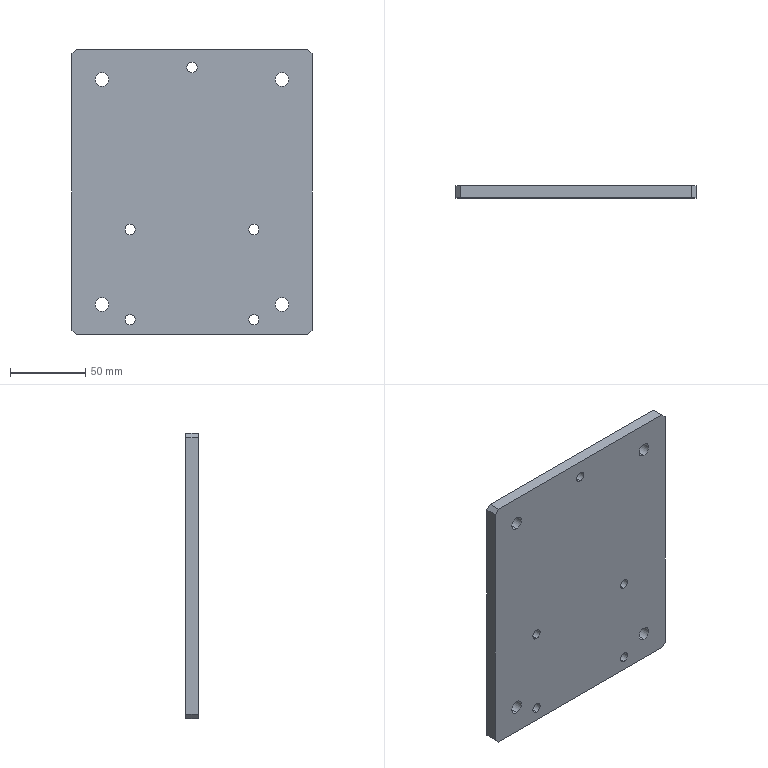Part | SolidWorks | features HoleWzd 3, Chamfer 1, Extrusion 1 | 1 solid | 28 faces | box 160 x 8 x 190 mm | volume 239568 mm3 | cylinder 18 | plane 10 | commonest cylinder face diameters 6.8 x10 9 x8
STEP:
#1=CARTESIAN_POINT('',(0.,4.,86.4));
#2=VERTEX_POINT('',#1);
#3=CARTESIAN_POINT('',(0.,4.,79.6));
#4=VERTEX_POINT('',#3);
#5=CARTESIAN_POINT('',(0.,4.,83.));
#6=DIRECTION('',(0.,-1.,0.));
#7=DIRECTION('',(0.,0.,-1.));
#8=AXIS2_PLACEMENT_3D('',#5,#6,#7);
#9=CIRCLE('',#8,3.4);
#10=EDGE_CURVE('',#2,#4,#9,.T.);
#11=ORIENTED_EDGE('',*,*,#10,.F.);
#12=CARTESIAN_POINT('',(0.,-4.,86.4));
#13=VERTEX_POINT('',#12);
#14=CARTESIAN_POINT('',(0.,-4.,86.4));
#15=DIRECTION('',(0.,-1.,0.));
#16=VECTOR('',#15,1000.);
#17=LINE('',#14,#16);
#18=EDGE_CURVE('',#2,#13,#17,.T.);
#19=ORIENTED_EDGE('',*,*,#18,.T.);
#20=CARTESIAN_POINT('',(0.,-4.,79.6));
#21=VERTEX_POINT('',#20);
#22=CARTESIAN_POINT('',(0.,-4.,83.));
#23=DIRECTION('',(0.,-1.,0.));
#24=DIRECTION('',(0.,0.,-1.));
#25=AXIS2_PLACEMENT_3D('',#22,#23,#24);
#26=CIRCLE('',#25,3.4);
#27=EDGE_CURVE('',#13,#21,#26,.T.);
#28=ORIENTED_EDGE('',*,*,#27,.T.);
#29=CARTESIAN_POINT('',(0.,-4.,79.6));
#30=DIRECTION('',(0.,-1.,0.));
#31=VECTOR('',#30,1000.);
#32=LINE('',#29,#31);
#33=EDGE_CURVE('',#4,#21,#32,.T.);
#34=ORIENTED_EDGE('',*,*,#33,.F.);
#35=EDGE_LOOP('',(#11,#19,#28,#34));
#36=FACE_OUTER_BOUND('',#35,.T.);
#37=CARTESIAN_POINT('',(0.,-4.,83.));
#38=DIRECTION('',(0.,-1.,0.));
#39=DIRECTION('',(0.,0.,-1.));
#40=AXIS2_PLACEMENT_3D('',#37,#38,#39);
#41=CYLINDRICAL_SURFACE('',#40,3.4);
#42=ADVANCED_FACE('',(#36),#41,.F.);
#43=CARTESIAN_POINT('',(41.25,4.,-21.6));
#44=VERTEX_POINT('',#43);
#45=CARTESIAN_POINT('',(41.25,4.,-28.4));
#46=VERTEX_POINT('',#45);
#47=CARTESIAN_POINT('',(41.25,4.,-25.));
#48=DIRECTION('',(0.,-1.,0.));
#49=DIRECTION('',(0.,0.,-1.));
#50=AXIS2_PLACEMENT_3D('',#47,#48,#49);
#51=CIRCLE('',#50,3.4);
#52=EDGE_CURVE('',#44,#46,#51,.T.);
#53=ORIENTED_EDGE('',*,*,#52,.F.);
#54=CARTESIAN_POINT('',(41.25,-4.,-21.6));
#55=VERTEX_POINT('',#54);
#56=CARTESIAN_POINT('',(41.25,-4.,-21.6));
#57=DIRECTION('',(0.,-1.,0.));
#58=VECTOR('',#57,1000.);
#59=LINE('',#56,#58);
#60=EDGE_CURVE('',#44,#55,#59,.T.);
#61=ORIENTED_EDGE('',*,*,#60,.T.);
#62=CARTESIAN_POINT('',(41.25,-4.,-28.4));
#63=VERTEX_POINT('',#62);
#64=CARTESIAN_POINT('',(41.25,-4.,-25.));
#65=DIRECTION('',(0.,-1.,0.));
#66=DIRECTION('',(0.,0.,-1.));
#67=AXIS2_PLACEMENT_3D('',#64,#65,#66);
#68=CIRCLE('',#67,3.4);
#69=EDGE_CURVE('',#55,#63,#68,.T.);
#70=ORIENTED_EDGE('',*,*,#69,.T.);
#71=CARTESIAN_POINT('',(41.25,-4.,-28.4));
#72=DIRECTION('',(0.,-1.,0.));
#73=VECTOR('',#72,1000.);
#74=LINE('',#71,#73);
#75=EDGE_CURVE('',#46,#63,#74,.T.);
#76=ORIENTED_EDGE('',*,*,#75,.F.);
#77=EDGE_LOOP('',(#53,#61,#70,#76));
#78=FACE_OUTER_BOUND('',#77,.T.);
#79=CARTESIAN_POINT('',(41.25,-4.,-25.));
#80=DIRECTION('',(0.,-1.,0.));
#81=DIRECTION('',(0.,0.,-1.));
#82=AXIS2_PLACEMENT_3D('',#79,#80,#81);
#83=CYLINDRICAL_SURFACE('',#82,3.4);
#84=ADVANCED_FACE('',(#78),#83,.F.);
#85=CARTESIAN_POINT('',(41.25,4.,-81.6));
#86=VERTEX_POINT('',#85);
#87=CARTESIAN_POINT('',(41.25,4.,-88.4));
#88=VERTEX_POINT('',#87);
#89=CARTESIAN_POINT('',(41.25,4.,-85.));
#90=DIRECTION('',(0.,-1.,0.));
#91=DIRECTION('',(0.,0.,-1.));
#92=AXIS2_PLACEMENT_3D('',#89,#90,#91);
#93=CIRCLE('',#92,3.4);
#94=EDGE_CURVE('',#86,#88,#93,.T.);
#95=ORIENTED_EDGE('',*,*,#94,.F.);
#96=CARTESIAN_POINT('',(41.25,-4.,-81.6));
#97=VERTEX_POINT('',#96);
#98=CARTESIAN_POINT('',(41.25,-4.,-81.6));
#99=DIRECTION('',(0.,-1.,0.));
#100=VECTOR('',#99,1000.);
#101=LINE('',#98,#100);
#102=EDGE_CURVE('',#86,#97,#101,.T.);
#103=ORIENTED_EDGE('',*,*,#102,.T.);
#104=CARTESIAN_POINT('',(41.25,-4.,-88.4));
#105=VERTEX_POINT('',#104);
#106=CARTESIAN_POINT('',(41.25,-4.,-85.));
#107=DIRECTION('',(0.,-1.,0.));
#108=DIRECTION('',(0.,0.,-1.));
#109=AXIS2_PLACEMENT_3D('',#106,#107,#108);
#110=CIRCLE('',#109,3.4);
#111=EDGE_CURVE('',#97,#105,#110,.T.);
#112=ORIENTED_EDGE('',*,*,#111,.T.);
#113=CARTESIAN_POINT('',(41.25,-4.,-88.4));
#114=DIRECTION('',(0.,-1.,0.));
#115=VECTOR('',#114,1000.);
#116=LINE('',#113,#115);
#117=EDGE_CURVE('',#88,#105,#116,.T.);
#118=ORIENTED_EDGE('',*,*,#117,.F.);
#119=EDGE_LOOP('',(#95,#103,#112,#118));
#120=FACE_OUTER_BOUND('',#119,.T.);
#121=CARTESIAN_POINT('',(41.25,-4.,-85.));
#122=DIRECTION('',(0.,-1.,0.));
#123=DIRECTION('',(0.,0.,-1.));
#124=AXIS2_PLACEMENT_3D('',#121,#122,#123);
#125=CYLINDRICAL_SURFACE('',#124,3.4);
#126=ADVANCED_FACE('',(#120),#125,.F.);
#127=CARTESIAN_POINT('',(-41.25,4.,-81.6));
#128=VERTEX_POINT('',#127);
#129=CARTESIAN_POINT('',(-41.25,4.,-88.4));
#130=VERTEX_POINT('',#129);
#131=CARTESIAN_POINT('',(-41.25,4.,-85.));
#132=DIRECTION('',(0.,-1.,0.));
#133=DIRECTION('',(0.,0.,-1.));
#134=AXIS2_PLACEMENT_3D('',#131,#132,#133);
#135=CIRCLE('',#134,3.4);
#136=EDGE_CURVE('',#128,#130,#135,.T.);
#137=ORIENTED_EDGE('',*,*,#136,.F.);
#138=CARTESIAN_POINT('',(-41.25,-4.,-81.6));
#139=VERTEX_POINT('',#138);
#140=CARTESIAN_POINT('',(-41.25,-4.,-81.6));
#141=DIRECTION('',(0.,-1.,0.));
#142=VECTOR('',#141,1000.);
#143=LINE('',#140,#142);
#144=EDGE_CURVE('',#128,#139,#143,.T.);
#145=ORIENTED_EDGE('',*,*,#144,.T.);
#146=CARTESIAN_POINT('',(-41.25,-4.,-88.4));
#147=VERTEX_POINT('',#146);
#148=CARTESIAN_POINT('',(-41.25,-4.,-85.));
#149=DIRECTION('',(0.,-1.,0.));
#150=DIRECTION('',(0.,0.,-1.));
#151=AXIS2_PLACEMENT_3D('',#148,#149,#150);
#152=CIRCLE('',#151,3.4);
#153=EDGE_CURVE('',#139,#147,#152,.T.);
#154=ORIENTED_EDGE('',*,*,#153,.T.);
#155=CARTESIAN_POINT('',(-41.25,-4.,-88.4));
#156=DIRECTION('',(0.,-1.,0.));
#157=VECTOR('',#156,1000.);
#158=LINE('',#155,#157);
#159=EDGE_CURVE('',#130,#147,#158,.T.);
#160=ORIENTED_EDGE('',*,*,#159,.F.);
#161=EDGE_LOOP('',(#137,#145,#154,#160));
#162=FACE_OUTER_BOUND('',#161,.T.);
#163=CARTESIAN_POINT('',(-41.25,-4.,-85.));
#164=DIRECTION('',(0.,-1.,0.));
#165=DIRECTION('',(0.,0.,-1.));
#166=AXIS2_PLACEMENT_3D('',#163,#164,#165);
#167=CYLINDRICAL_SURFACE('',#166,3.4);
#168=ADVANCED_FACE('',(#162),#167,.F.);
#169=CARTESIAN_POINT('',(-41.25,4.,-21.6));
#170=VERTEX_POINT('',#169);
#171=CARTESIAN_POINT('',(-41.25,4.,-28.4));
#172=VERTEX_POINT('',#171);
#173=CARTESIAN_POINT('',(-41.25,4.,-25.));
#174=DIRECTION('',(0.,-1.,0.));
#175=DIRECTION('',(0.,0.,-1.));
#176=AXIS2_PLACEMENT_3D('',#173,#174,#175);
#177=CIRCLE('',#176,3.4);
#178=EDGE_CURVE('',#170,#172,#177,.T.);
#179=ORIENTED_EDGE('',*,*,#178,.F.);
#180=CARTESIAN_POINT('',(-41.25,-4.,-21.6));
#181=VERTEX_POINT('',#180);
#182=CARTESIAN_POINT('',(-41.25,-4.,-21.6));
#183=DIRECTION('',(0.,-1.,0.));
#184=VECTOR('',#183,1000.);
#185=LINE('',#182,#184);
#186=EDGE_CURVE('',#170,#181,#185,.T.);
#187=ORIENTED_EDGE('',*,*,#186,.T.);
#188=CARTESIAN_POINT('',(-41.25,-4.,-28.4));
#189=VERTEX_POINT('',#188);
#190=CARTESIAN_POINT('',(-41.25,-4.,-25.));
#191=DIRECTION('',(0.,-1.,0.));
#192=DIRECTION('',(0.,0.,-1.));
#193=AXIS2_PLACEMENT_3D('',#190,#191,#192);
#194=CIRCLE('',#193,3.4);
#195=EDGE_CURVE('',#181,#189,#194,.T.);
#196=ORIENTED_EDGE('',*,*,#195,.T.);
#197=CARTESIAN_POINT('',(-41.25,-4.,-28.4));
#198=DIRECTION('',(0.,-1.,0.));
#199=VECTOR('',#198,1000.);
#200=LINE('',#197,#199);
#201=EDGE_CURVE('',#172,#189,#200,.T.);
#202=ORIENTED_EDGE('',*,*,#201,.F.);
#203=EDGE_LOOP('',(#179,#187,#196,#202));
#204=FACE_OUTER_BOUND('',#203,.T.);
#205=CARTESIAN_POINT('',(-41.25,-4.,-25.));
#206=DIRECTION('',(0.,-1.,0.));
#207=DIRECTION('',(0.,0.,-1.));
#208=AXIS2_PLACEMENT_3D('',#205,#206,#207);
#209=CYLINDRICAL_SURFACE('',#208,3.4);
#210=ADVANCED_FACE('',(#204),#209,.F.);
#211=CARTESIAN_POINT('',(60.,4.,79.5));
#212=VERTEX_POINT('',#211);
#213=CARTESIAN_POINT('',(60.,4.,70.5));
#214=VERTEX_POINT('',#213);
#215=CARTESIAN_POINT('',(60.,4.,75.));
#216=DIRECTION('',(0.,-1.,0.));
#217=DIRECTION('',(0.,0.,-1.));
#218=AXIS2_PLACEMENT_3D('',#215,#216,#217);
#219=CIRCLE('',#218,4.5);
#220=EDGE_CURVE('',#212,#214,#219,.T.);
#221=ORIENTED_EDGE('',*,*,#220,.F.);
#222=CARTESIAN_POINT('',(60.,-4.,79.5));
#223=VERTEX_POINT('',#222);
#224=CARTESIAN_POINT('',(60.,-4.,79.5));
#225=DIRECTION('',(0.,-1.,0.));
#226=VECTOR('',#225,1000.);
#227=LINE('',#224,#226);
#228=EDGE_CURVE('',#212,#223,#227,.T.);
#229=ORIENTED_EDGE('',*,*,#228,.T.);
#230=CARTESIAN_POINT('',(60.,-4.,70.5));
#231=VERTEX_POINT('',#230);
#232=CARTESIAN_POINT('',(60.,-4.,75.));
#233=DIRECTION('',(0.,-1.,0.));
#234=DIRECTION('',(0.,0.,-1.));
#235=AXIS2_PLACEMENT_3D('',#232,#233,#234);
#236=CIRCLE('',#235,4.5);
#237=EDGE_CURVE('',#223,#231,#236,.T.);
#238=ORIENTED_EDGE('',*,*,#237,.T.);
#239=CARTESIAN_POINT('',(60.,-4.,70.5));
#240=DIRECTION('',(0.,-1.,0.));
#241=VECTOR('',#240,1000.);
#242=LINE('',#239,#241);
#243=EDGE_CURVE('',#214,#231,#242,.T.);
#244=ORIENTED_EDGE('',*,*,#243,.F.);
#245=EDGE_LOOP('',(#221,#229,#238,#244));
#246=FACE_OUTER_BOUND('',#245,.T.);
#247=CARTESIAN_POINT('',(60.,-4.,75.));
#248=DIRECTION('',(0.,-1.,0.));
#249=DIRECTION('',(0.,0.,-1.));
#250=AXIS2_PLACEMENT_3D('',#247,#248,#249);
#251=CYLINDRICAL_SURFACE('',#250,4.5);
#252=ADVANCED_FACE('',(#246),#251,.F.);
#253=CARTESIAN_POINT('',(-60.,4.,79.5));
#254=VERTEX_POINT('',#253);
#255=CARTESIAN_POINT('',(-60.,4.,70.5));
#256=VERTEX_POINT('',#255);
#257=CARTESIAN_POINT('',(-60.,4.,75.));
#258=DIRECTION('',(0.,-1.,0.));
#259=DIRECTION('',(0.,0.,-1.));
#260=AXIS2_PLACEMENT_3D('',#257,#258,#259);
#261=CIRCLE('',#260,4.5);
#262=EDGE_CURVE('',#254,#256,#261,.T.);
#263=ORIENTED_EDGE('',*,*,#262,.F.);
#264=CARTESIAN_POINT('',(-60.,-4.,79.5));
#265=VERTEX_POINT('',#264);
#266=CARTESIAN_POINT('',(-60.,-4.,79.5));
#267=DIRECTION('',(0.,-1.,0.));
#268=VECTOR('',#267,1000.);
#269=LINE('',#266,#268);
#270=EDGE_CURVE('',#254,#265,#269,.T.);
#271=ORIENTED_EDGE('',*,*,#270,.T.);
#272=CARTESIAN_POINT('',(-60.,-4.,70.5));
#273=VERTEX_POINT('',#272);
#274=CARTESIAN_POINT('',(-60.,-4.,75.));
#275=DIRECTION('',(0.,-1.,0.));
#276=DIRECTION('',(0.,0.,-1.));
#277=AXIS2_PLACEMENT_3D('',#274,#275,#276);
#278=CIRCLE('',#277,4.5);
#279=EDGE_CURVE('',#265,#273,#278,.T.);
#280=ORIENTED_EDGE('',*,*,#279,.T.);
#281=CARTESIAN_POINT('',(-60.,-4.,70.5));
#282=DIRECTION('',(0.,-1.,0.));
#283=VECTOR('',#282,1000.);
#284=LINE('',#281,#283);
#285=EDGE_CURVE('',#256,#273,#284,.T.);
#286=ORIENTED_EDGE('',*,*,#285,.F.);
#287=EDGE_LOOP('',(#263,#271,#280,#286));
#288=FACE_OUTER_BOUND('',#287,.T.);
#289=CARTESIAN_POINT('',(-60.,-4.,75.));
#290=DIRECTION('',(0.,-1.,0.));
#291=DIRECTION('',(0.,0.,-1.));
#292=AXIS2_PLACEMENT_3D('',#289,#290,#291);
#293=CYLINDRICAL_SURFACE('',#292,4.5);
#294=ADVANCED_FACE('',(#288),#293,.F.);
#295=CARTESIAN_POINT('',(-60.,4.,-70.5));
#296=VERTEX_POINT('',#295);
#297=CARTESIAN_POINT('',(-60.,4.,-79.5));
#298=VERTEX_POINT('',#297);
#299=CARTESIAN_POINT('',(-60.,4.,-75.));
#300=DIRECTION('',(0.,-1.,0.));
#301=DIRECTION('',(0.,0.,-1.));
#302=AXIS2_PLACEMENT_3D('',#299,#300,#301);
#303=CIRCLE('',#302,4.5);
#304=EDGE_CURVE('',#296,#298,#303,.T.);
#305=ORIENTED_EDGE('',*,*,#304,.F.);
#306=CARTESIAN_POINT('',(-60.,-4.,-70.5));
#307=VERTEX_POINT('',#306);
#308=CARTESIAN_POINT('',(-60.,-4.,-70.5));
#309=DIRECTION('',(0.,-1.,0.));
#310=VECTOR('',#309,1000.);
#311=LINE('',#308,#310);
#312=EDGE_CURVE('',#296,#307,#311,.T.);
#313=ORIENTED_EDGE('',*,*,#312,.T.);
#314=CARTESIAN_POINT('',(-60.,-4.,-79.5));
#315=VERTEX_POINT('',#314);
#316=CARTESIAN_POINT('',(-60.,-4.,-75.));
#317=DIRECTION('',(0.,-1.,0.));
#318=DIRECTION('',(0.,0.,-1.));
#319=AXIS2_PLACEMENT_3D('',#316,#317,#318);
#320=CIRCLE('',#319,4.5);
#321=EDGE_CURVE('',#307,#315,#320,.T.);
#322=ORIENTED_EDGE('',*,*,#321,.T.);
#323=CARTESIAN_POINT('',(-60.,-4.,-79.5));
#324=DIRECTION('',(0.,-1.,0.));
#325=VECTOR('',#324,1000.);
#326=LINE('',#323,#325);
#327=EDGE_CURVE('',#298,#315,#326,.T.);
#328=ORIENTED_EDGE('',*,*,#327,.F.);
#329=EDGE_LOOP('',(#305,#313,#322,#328));
#330=FACE_OUTER_BOUND('',#329,.T.);
#331=CARTESIAN_POINT('',(-60.,-4.,-75.));
#332=DIRECTION('',(0.,-1.,0.));
#333=DIRECTION('',(0.,0.,-1.));
#334=AXIS2_PLACEMENT_3D('',#331,#332,#333);
#335=CYLINDRICAL_SURFACE('',#334,4.5);
#336=ADVANCED_FACE('',(#330),#335,.F.);
#337=CARTESIAN_POINT('',(60.,4.,-70.5));
#338=VERTEX_POINT('',#337);
#339=CARTESIAN_POINT('',(60.,4.,-79.5));
#340=VERTEX_POINT('',#339);
#341=CARTESIAN_POINT('',(60.,4.,-75.));
#342=DIRECTION('',(0.,-1.,0.));
#343=DIRECTION('',(0.,0.,-1.));
#344=AXIS2_PLACEMENT_3D('',#341,#342,#343);
#345=CIRCLE('',#344,4.5);
#346=EDGE_CURVE('',#338,#340,#345,.T.);
#347=ORIENTED_EDGE('',*,*,#346,.F.);
#348=CARTESIAN_POINT('',(60.,-4.,-70.5));
#349=VERTEX_POINT('',#348);
#350=CARTESIAN_POINT('',(60.,-4.,-70.5));
#351=DIRECTION('',(0.,-1.,0.));
#352=VECTOR('',#351,1000.);
#353=LINE('',#350,#352);
#354=EDGE_CURVE('',#338,#349,#353,.T.);
#355=ORIENTED_EDGE('',*,*,#354,.T.);
#356=CARTESIAN_POINT('',(60.,-4.,-79.5));
#357=VERTEX_POINT('',#356);
#358=CARTESIAN_POINT('',(60.,-4.,-75.));
#359=DIRECTION('',(0.,-1.,0.));
#360=DIRECTION('',(0.,0.,-1.));
#361=AXIS2_PLACEMENT_3D('',#358,#359,#360);
#362=CIRCLE('',#361,4.5);
#363=EDGE_CURVE('',#349,#357,#362,.T.);
#364=ORIENTED_EDGE('',*,*,#363,.T.);
#365=CARTESIAN_POINT('',(60.,-4.,-79.5));
#366=DIRECTION('',(0.,-1.,0.));
#367=VECTOR('',#366,1000.);
#368=LINE('',#365,#367);
#369=EDGE_CURVE('',#340,#357,#368,.T.);
#370=ORIENTED_EDGE('',*,*,#369,.F.);
#371=EDGE_LOOP('',(#347,#355,#364,#370));
#372=FACE_OUTER_BOUND('',#371,.T.);
#373=CARTESIAN_POINT('',(60.,-4.,-75.));
#374=DIRECTION('',(0.,-1.,0.));
#375=DIRECTION('',(0.,0.,-1.));
#376=AXIS2_PLACEMENT_3D('',#373,#374,#375);
#377=CYLINDRICAL_SURFACE('',#376,4.5);
#378=ADVANCED_FACE('',(#372),#377,.F.);
#379=CARTESIAN_POINT('',(80.,-4.,92.));
#380=VERTEX_POINT('',#379);
#381=CARTESIAN_POINT('',(80.,-4.,-92.));
#382=VERTEX_POINT('',#381);
#383=CARTESIAN_POINT('',(80.,-4.,95.));
#384=DIRECTION('',(0.,0.,-1.));
#385=VECTOR('',#384,1000.);
#386=LINE('',#383,#385);
#387=EDGE_CURVE('',#380,#382,#386,.T.);
#388=ORIENTED_EDGE('',*,*,#387,.T.);
#389=CARTESIAN_POINT('',(80.,4.,-92.));
#390=VERTEX_POINT('',#389);
#391=CARTESIAN_POINT('',(80.,4.,-92.));
#392=DIRECTION('',(0.,1.,0.));
#393=VECTOR('',#392,1000.);
#394=LINE('',#391,#393);
#395=EDGE_CURVE('',#382,#390,#394,.T.);
#396=ORIENTED_EDGE('',*,*,#395,.T.);
#397=CARTESIAN_POINT('',(80.,4.,92.));
#398=VERTEX_POINT('',#397);
#399=CARTESIAN_POINT('',(80.,4.,95.));
#400=DIRECTION('',(0.,0.,-1.));
#401=VECTOR('',#400,1000.);
#402=LINE('',#399,#401);
#403=EDGE_CURVE('',#398,#390,#402,.T.);
#404=ORIENTED_EDGE('',*,*,#403,.F.);
#405=CARTESIAN_POINT('',(80.,4.,92.));
#406=DIRECTION('',(0.,-1.,0.));
#407=VECTOR('',#406,1000.);
#408=LINE('',#405,#407);
#409=EDGE_CURVE('',#398,#380,#408,.T.);
#410=ORIENTED_EDGE('',*,*,#409,.T.);
#411=EDGE_LOOP('',(#388,#396,#404,#410));
#412=FACE_OUTER_BOUND('',#411,.T.);
#413=CARTESIAN_POINT('',(80.,4.,95.));
#414=DIRECTION('',(-1.,0.,0.));
#415=DIRECTION('',(0.,0.,1.));
#416=AXIS2_PLACEMENT_3D('',#413,#414,#415);
#417=PLANE('',#416);
#418=ADVANCED_FACE('',(#412),#417,.F.);
#419=CARTESIAN_POINT('',(77.,4.,-95.));
#420=VERTEX_POINT('',#419);
#421=CARTESIAN_POINT('',(-77.,4.,-95.));
#422=VERTEX_POINT('',#421);
#423=CARTESIAN_POINT('',(-80.,4.,-95.));
#424=DIRECTION('',(-1.,0.,0.));
#425=VECTOR('',#424,1000.);
#426=LINE('',#423,#425);
#427=EDGE_CURVE('',#420,#422,#426,.T.);
#428=ORIENTED_EDGE('',*,*,#427,.F.);
#429=CARTESIAN_POINT('',(77.,-4.,-95.));
#430=VERTEX_POINT('',#429);
#431=CARTESIAN_POINT('',(77.,4.,-95.));
#432=DIRECTION('',(0.,-1.,0.));
#433=VECTOR('',#432,1000.);
#434=LINE('',#431,#433);
#435=EDGE_CURVE('',#420,#430,#434,.T.);
#436=ORIENTED_EDGE('',*,*,#435,.T.);
#437=CARTESIAN_POINT('',(-77.,-4.,-95.));
#438=VERTEX_POINT('',#437);
#439=CARTESIAN_POINT('',(-80.,-4.,-95.));
#440=DIRECTION('',(-1.,0.,0.));
#441=VECTOR('',#440,1000.);
#442=LINE('',#439,#441);
#443=EDGE_CURVE('',#430,#438,#442,.T.);
#444=ORIENTED_EDGE('',*,*,#443,.T.);
#445=CARTESIAN_POINT('',(-77.,4.,-95.));
#446=DIRECTION('',(0.,1.,0.));
#447=VECTOR('',#446,1000.);
#448=LINE('',#445,#447);
#449=EDGE_CURVE('',#438,#422,#448,.T.);
#450=ORIENTED_EDGE('',*,*,#449,.T.);
#451=EDGE_LOOP('',(#428,#436,#444,#450));
#452=FACE_OUTER_BOUND('',#451,.T.);
#453=CARTESIAN_POINT('',(-80.,4.,-95.));
#454=DIRECTION('',(0.,0.,1.));
#455=DIRECTION('',(1.,0.,0.));
#456=AXIS2_PLACEMENT_3D('',#453,#454,#455);
#457=PLANE('',#456);
#458=ADVANCED_FACE('',(#452),#457,.F.);
#459=CARTESIAN_POINT('',(-80.,4.,-92.));
#460=VERTEX_POINT('',#459);
#461=CARTESIAN_POINT('',(-80.,4.,92.));
#462=VERTEX_POINT('',#461);
#463=CARTESIAN_POINT('',(-80.,4.,95.));
#464=DIRECTION('',(0.,0.,1.));
#465=VECTOR('',#464,1000.);
#466=LINE('',#463,#465);
#467=EDGE_CURVE('',#460,#462,#466,.T.);
#468=ORIENTED_EDGE('',*,*,#467,.F.);
#469=CARTESIAN_POINT('',(-80.,-4.,-92.));
#470=VERTEX_POINT('',#469);
#471=CARTESIAN_POINT('',(-80.,4.,-92.));
#472=DIRECTION('',(0.,-1.,0.));
#473=VECTOR('',#472,1000.);
#474=LINE('',#471,#473);
#475=EDGE_CURVE('',#460,#470,#474,.T.);
#476=ORIENTED_EDGE('',*,*,#475,.T.);
#477=CARTESIAN_POINT('',(-80.,-4.,92.));
#478=VERTEX_POINT('',#477);
#479=CARTESIAN_POINT('',(-80.,-4.,95.));
#480=DIRECTION('',(0.,0.,1.));
#481=VECTOR('',#480,1000.);
#482=LINE('',#479,#481);
#483=EDGE_CURVE('',#470,#478,#482,.T.);
#484=ORIENTED_EDGE('',*,*,#483,.T.);
#485=CARTESIAN_POINT('',(-80.,4.,92.));
#486=DIRECTION('',(0.,1.,0.));
#487=VECTOR('',#486,1000.);
#488=LINE('',#485,#487);
#489=EDGE_CURVE('',#478,#462,#488,.T.);
#490=ORIENTED_EDGE('',*,*,#489,.T.);
#491=EDGE_LOOP('',(#468,#476,#484,#490));
#492=FACE_OUTER_BOUND('',#491,.T.);
#493=CARTESIAN_POINT('',(-80.,4.,95.));
#494=DIRECTION('',(1.,0.,0.));
#495=DIRECTION('',(0.,0.,-1.));
#496=AXIS2_PLACEMENT_3D('',#493,#494,#495);
#497=PLANE('',#496);
#498=ADVANCED_FACE('',(#492),#497,.F.);
#499=CARTESIAN_POINT('',(-77.,-4.,95.));
#500=VERTEX_POINT('',#499);
#501=CARTESIAN_POINT('',(77.,-4.,95.));
#502=VERTEX_POINT('',#501);
#503=CARTESIAN_POINT('',(-80.,-4.,95.));
#504=DIRECTION('',(1.,0.,0.));
#505=VECTOR('',#504,1000.);
#506=LINE('',#503,#505);
#507=EDGE_CURVE('',#500,#502,#506,.T.);
#508=ORIENTED_EDGE('',*,*,#507,.T.);
#509=CARTESIAN_POINT('',(77.,4.,95.));
#510=VERTEX_POINT('',#509);
#511=CARTESIAN_POINT('',(77.,4.,95.));
#512=DIRECTION('',(0.,1.,0.));
#513=VECTOR('',#512,1000.);
#514=LINE('',#511,#513);
#515=EDGE_CURVE('',#502,#510,#514,.T.);
#516=ORIENTED_EDGE('',*,*,#515,.T.);
#517=CARTESIAN_POINT('',(-77.,4.,95.));
#518=VERTEX_POINT('',#517);
#519=CARTESIAN_POINT('',(-80.,4.,95.));
#520=DIRECTION('',(1.,0.,0.));
#521=VECTOR('',#520,1000.);
#522=LINE('',#519,#521);
#523=EDGE_CURVE('',#518,#510,#522,.T.);
#524=ORIENTED_EDGE('',*,*,#523,.F.);
#525=CARTESIAN_POINT('',(-77.,4.,95.));
#526=DIRECTION('',(0.,-1.,0.));
#527=VECTOR('',#526,1000.);
#528=LINE('',#525,#527);
#529=EDGE_CURVE('',#518,#500,#528,.T.);
#530=ORIENTED_EDGE('',*,*,#529,.T.);
#531=EDGE_LOOP('',(#508,#516,#524,#530));
#532=FACE_OUTER_BOUND('',#531,.T.);
#533=CARTESIAN_POINT('',(-80.,4.,95.));
#534=DIRECTION('',(0.,0.,-1.));
#535=DIRECTION('',(-1.,0.,0.));
#536=AXIS2_PLACEMENT_3D('',#533,#534,#535);
#537=PLANE('',#536);
#538=ADVANCED_FACE('',(#532),#537,.F.);
#539=CARTESIAN_POINT('',(0.,4.,83.));
#540=DIRECTION('',(0.,-1.,0.));
#541=DIRECTION('',(0.,0.,-1.));
#542=AXIS2_PLACEMENT_3D('',#539,#540,#541);
#543=CIRCLE('',#542,3.4);
#544=EDGE_CURVE('',#4,#2,#543,.T.);
#545=ORIENTED_EDGE('',*,*,#544,.T.);
#546=ORIENTED_EDGE('',*,*,#10,.T.);
#547=EDGE_LOOP('',(#545,#546));
#548=FACE_BOUND('',#547,.T.);
#549=CARTESIAN_POINT('',(41.25,4.,-25.));
#550=DIRECTION('',(0.,-1.,0.));
#551=DIRECTION('',(0.,0.,-1.));
#552=AXIS2_PLACEMENT_3D('',#549,#550,#551);
#553=CIRCLE('',#552,3.4);
#554=EDGE_CURVE('',#46,#44,#553,.T.);
#555=ORIENTED_EDGE('',*,*,#554,.T.);
#556=ORIENTED_EDGE('',*,*,#52,.T.);
#557=EDGE_LOOP('',(#555,#556));
#558=FACE_BOUND('',#557,.T.);
#559=CARTESIAN_POINT('',(41.25,4.,-85.));
#560=DIRECTION('',(0.,-1.,0.));
#561=DIRECTION('',(0.,0.,-1.));
#562=AXIS2_PLACEMENT_3D('',#559,#560,#561);
#563=CIRCLE('',#562,3.4);
#564=EDGE_CURVE('',#88,#86,#563,.T.);
#565=ORIENTED_EDGE('',*,*,#564,.T.);
#566=ORIENTED_EDGE('',*,*,#94,.T.);
#567=EDGE_LOOP('',(#565,#566));
#568=FACE_BOUND('',#567,.T.);
#569=CARTESIAN_POINT('',(-41.25,4.,-85.));
#570=DIRECTION('',(0.,-1.,0.));
#571=DIRECTION('',(0.,0.,-1.));
#572=AXIS2_PLACEMENT_3D('',#569,#570,#571);
#573=CIRCLE('',#572,3.4);
#574=EDGE_CURVE('',#130,#128,#573,.T.);
#575=ORIENTED_EDGE('',*,*,#574,.T.);
#576=ORIENTED_EDGE('',*,*,#136,.T.);
#577=EDGE_LOOP('',(#575,#576));
#578=FACE_BOUND('',#577,.T.);
#579=CARTESIAN_POINT('',(-41.25,4.,-25.));
#580=DIRECTION('',(0.,-1.,0.));
#581=DIRECTION('',(0.,0.,-1.));
#582=AXIS2_PLACEMENT_3D('',#579,#580,#581);
#583=CIRCLE('',#582,3.4);
#584=EDGE_CURVE('',#172,#170,#583,.T.);
#585=ORIENTED_EDGE('',*,*,#584,.T.);
#586=ORIENTED_EDGE('',*,*,#178,.T.);
#587=EDGE_LOOP('',(#585,#586));
#588=FACE_BOUND('',#587,.T.);
#589=CARTESIAN_POINT('',(60.,4.,75.));
#590=DIRECTION('',(0.,-1.,0.));
#591=DIRECTION('',(0.,0.,-1.));
#592=AXIS2_PLACEMENT_3D('',#589,#590,#591);
#593=CIRCLE('',#592,4.5);
#594=EDGE_CURVE('',#214,#212,#593,.T.);
#595=ORIENTED_EDGE('',*,*,#594,.T.);
#596=ORIENTED_EDGE('',*,*,#220,.T.);
#597=EDGE_LOOP('',(#595,#596));
#598=FACE_BOUND('',#597,.T.);
#599=CARTESIAN_POINT('',(-60.,4.,75.));
#600=DIRECTION('',(0.,-1.,0.));
#601=DIRECTION('',(0.,0.,-1.));
#602=AXIS2_PLACEMENT_3D('',#599,#600,#601);
#603=CIRCLE('',#602,4.5);
#604=EDGE_CURVE('',#256,#254,#603,.T.);
#605=ORIENTED_EDGE('',*,*,#604,.T.);
#606=ORIENTED_EDGE('',*,*,#262,.T.);
#607=EDGE_LOOP('',(#605,#606));
#608=FACE_BOUND('',#607,.T.);
#609=CARTESIAN_POINT('',(-60.,4.,-75.));
#610=DIRECTION('',(0.,-1.,0.));
#611=DIRECTION('',(0.,0.,-1.));
#612=AXIS2_PLACEMENT_3D('',#609,#610,#611);
#613=CIRCLE('',#612,4.5);
#614=EDGE_CURVE('',#298,#296,#613,.T.);
#615=ORIENTED_EDGE('',*,*,#614,.T.);
#616=ORIENTED_EDGE('',*,*,#304,.T.);
#617=EDGE_LOOP('',(#615,#616));
#618=FACE_BOUND('',#617,.T.);
#619=CARTESIAN_POINT('',(60.,4.,-75.));
#620=DIRECTION('',(0.,-1.,0.));
#621=DIRECTION('',(0.,0.,-1.));
#622=AXIS2_PLACEMENT_3D('',#619,#620,#621);
#623=CIRCLE('',#622,4.5);
#624=EDGE_CURVE('',#340,#338,#623,.T.);
#625=ORIENTED_EDGE('',*,*,#624,.T.);
#626=ORIENTED_EDGE('',*,*,#346,.T.);
#627=EDGE_LOOP('',(#625,#626));
#628=FACE_BOUND('',#627,.T.);
#629=ORIENTED_EDGE('',*,*,#403,.T.);
#630=CARTESIAN_POINT('',(77.,4.,-95.));
#631=DIRECTION('',(-0.7071,0.,-0.7071));
#632=VECTOR('',#631,1000.);
#633=LINE('',#630,#632);
#634=EDGE_CURVE('',#390,#420,#633,.T.);
#635=ORIENTED_EDGE('',*,*,#634,.T.);
#636=ORIENTED_EDGE('',*,*,#427,.T.);
#637=CARTESIAN_POINT('',(-80.,4.,-92.));
#638=DIRECTION('',(-0.7071,0.,0.7071));
#639=VECTOR('',#638,1000.);
#640=LINE('',#637,#639);
#641=EDGE_CURVE('',#422,#460,#640,.T.);
#642=ORIENTED_EDGE('',*,*,#641,.T.);
#643=ORIENTED_EDGE('',*,*,#467,.T.);
#644=CARTESIAN_POINT('',(-77.,4.,95.));
#645=DIRECTION('',(0.7071,0.,0.7071));
#646=VECTOR('',#645,1000.);
#647=LINE('',#644,#646);
#648=EDGE_CURVE('',#462,#518,#647,.T.);
#649=ORIENTED_EDGE('',*,*,#648,.T.);
#650=ORIENTED_EDGE('',*,*,#523,.T.);
#651=CARTESIAN_POINT('',(80.,4.,92.));
#652=DIRECTION('',(0.7071,0.,-0.7071));
#653=VECTOR('',#652,1000.);
#654=LINE('',#651,#653);
#655=EDGE_CURVE('',#510,#398,#654,.T.);
#656=ORIENTED_EDGE('',*,*,#655,.T.);
#657=EDGE_LOOP('',(#629,#635,#636,#642,#643,#649,#650,#656));
#658=FACE_OUTER_BOUND('',#657,.T.);
#659=CARTESIAN_POINT('',(0.,4.,0.));
#660=DIRECTION('',(0.,-1.,0.));
#661=DIRECTION('',(0.,0.,-1.));
#662=AXIS2_PLACEMENT_3D('',#659,#660,#661);
#663=PLANE('',#662);
#664=ADVANCED_FACE('',(#548,#558,#568,#578,#588,#598,#608,#618,#628,#658),#663,.F.);
#665=CARTESIAN_POINT('',(0.,-4.,83.));
#666=DIRECTION('',(0.,-1.,0.));
#667=DIRECTION('',(0.,0.,-1.));
#668=AXIS2_PLACEMENT_3D('',#665,#666,#667);
#669=CIRCLE('',#668,3.4);
#670=EDGE_CURVE('',#21,#13,#669,.T.);
#671=ORIENTED_EDGE('',*,*,#670,.F.);
#672=ORIENTED_EDGE('',*,*,#27,.F.);
#673=EDGE_LOOP('',(#671,#672));
#674=FACE_BOUND('',#673,.T.);
#675=CARTESIAN_POINT('',(41.25,-4.,-25.));
#676=DIRECTION('',(0.,-1.,0.));
#677=DIRECTION('',(0.,0.,-1.));
#678=AXIS2_PLACEMENT_3D('',#675,#676,#677);
#679=CIRCLE('',#678,3.4);
#680=EDGE_CURVE('',#63,#55,#679,.T.);
#681=ORIENTED_EDGE('',*,*,#680,.F.);
#682=ORIENTED_EDGE('',*,*,#69,.F.);
#683=EDGE_LOOP('',(#681,#682));
#684=FACE_BOUND('',#683,.T.);
#685=CARTESIAN_POINT('',(41.25,-4.,-85.));
#686=DIRECTION('',(0.,-1.,0.));
#687=DIRECTION('',(0.,0.,-1.));
#688=AXIS2_PLACEMENT_3D('',#685,#686,#687);
#689=CIRCLE('',#688,3.4);
#690=EDGE_CURVE('',#105,#97,#689,.T.);
#691=ORIENTED_EDGE('',*,*,#690,.F.);
#692=ORIENTED_EDGE('',*,*,#111,.F.);
#693=EDGE_LOOP('',(#691,#692));
#694=FACE_BOUND('',#693,.T.);
#695=CARTESIAN_POINT('',(-41.25,-4.,-85.));
#696=DIRECTION('',(0.,-1.,0.));
#697=DIRECTION('',(0.,0.,-1.));
#698=AXIS2_PLACEMENT_3D('',#695,#696,#697);
#699=CIRCLE('',#698,3.4);
#700=EDGE_CURVE('',#147,#139,#699,.T.);
#701=ORIENTED_EDGE('',*,*,#700,.F.);
#702=ORIENTED_EDGE('',*,*,#153,.F.);
#703=EDGE_LOOP('',(#701,#702));
#704=FACE_BOUND('',#703,.T.);
#705=CARTESIAN_POINT('',(-41.25,-4.,-25.));
#706=DIRECTION('',(0.,-1.,0.));
#707=DIRECTION('',(0.,0.,-1.));
#708=AXIS2_PLACEMENT_3D('',#705,#706,#707);
#709=CIRCLE('',#708,3.4);
#710=EDGE_CURVE('',#189,#181,#709,.T.);
#711=ORIENTED_EDGE('',*,*,#710,.F.);
#712=ORIENTED_EDGE('',*,*,#195,.F.);
#713=EDGE_LOOP('',(#711,#712));
#714=FACE_BOUND('',#713,.T.);
#715=CARTESIAN_POINT('',(60.,-4.,75.));
#716=DIRECTION('',(0.,-1.,0.));
#717=DIRECTION('',(0.,0.,-1.));
#718=AXIS2_PLACEMENT_3D('',#715,#716,#717);
#719=CIRCLE('',#718,4.5);
#720=EDGE_CURVE('',#231,#223,#719,.T.);
#721=ORIENTED_EDGE('',*,*,#720,.F.);
#722=ORIENTED_EDGE('',*,*,#237,.F.);
#723=EDGE_LOOP('',(#721,#722));
#724=FACE_BOUND('',#723,.T.);
#725=CARTESIAN_POINT('',(-60.,-4.,75.));
#726=DIRECTION('',(0.,-1.,0.));
#727=DIRECTION('',(0.,0.,-1.));
#728=AXIS2_PLACEMENT_3D('',#725,#726,#727);
#729=CIRCLE('',#728,4.5);
#730=EDGE_CURVE('',#273,#265,#729,.T.);
#731=ORIENTED_EDGE('',*,*,#730,.F.);
#732=ORIENTED_EDGE('',*,*,#279,.F.);
#733=EDGE_LOOP('',(#731,#732));
#734=FACE_BOUND('',#733,.T.);
#735=CARTESIAN_POINT('',(-60.,-4.,-75.));
#736=DIRECTION('',(0.,-1.,0.));
#737=DIRECTION('',(0.,0.,-1.));
#738=AXIS2_PLACEMENT_3D('',#735,#736,#737);
#739=CIRCLE('',#738,4.5);
#740=EDGE_CURVE('',#315,#307,#739,.T.);
#741=ORIENTED_EDGE('',*,*,#740,.F.);
#742=ORIENTED_EDGE('',*,*,#321,.F.);
#743=EDGE_LOOP('',(#741,#742));
#744=FACE_BOUND('',#743,.T.);
#745=CARTESIAN_POINT('',(60.,-4.,-75.));
#746=DIRECTION('',(0.,-1.,0.));
#747=DIRECTION('',(0.,0.,-1.));
#748=AXIS2_PLACEMENT_3D('',#745,#746,#747);
#749=CIRCLE('',#748,4.5);
#750=EDGE_CURVE('',#357,#349,#749,.T.);
#751=ORIENTED_EDGE('',*,*,#750,.F.);
#752=ORIENTED_EDGE('',*,*,#363,.F.);
#753=EDGE_LOOP('',(#751,#752));
#754=FACE_BOUND('',#753,.T.);
#755=ORIENTED_EDGE('',*,*,#443,.F.);
#756=CARTESIAN_POINT('',(86.,-4.,-86.));
#757=DIRECTION('',(0.7071,0.,0.7071));
#758=VECTOR('',#757,1000.);
#759=LINE('',#756,#758);
#760=EDGE_CURVE('',#430,#382,#759,.T.);
#761=ORIENTED_EDGE('',*,*,#760,.T.);
#762=ORIENTED_EDGE('',*,*,#387,.F.);
#763=CARTESIAN_POINT('',(86.,-4.,86.));
#764=DIRECTION('',(-0.7071,0.,0.7071));
#765=VECTOR('',#764,1000.);
#766=LINE('',#763,#765);
#767=EDGE_CURVE('',#380,#502,#766,.T.);
#768=ORIENTED_EDGE('',*,*,#767,.T.);
#769=ORIENTED_EDGE('',*,*,#507,.F.);
#770=CARTESIAN_POINT('',(-86.,-4.,86.));
#771=DIRECTION('',(-0.7071,0.,-0.7071));
#772=VECTOR('',#771,1000.);
#773=LINE('',#770,#772);
#774=EDGE_CURVE('',#500,#478,#773,.T.);
#775=ORIENTED_EDGE('',*,*,#774,.T.);
#776=ORIENTED_EDGE('',*,*,#483,.F.);
#777=CARTESIAN_POINT('',(-86.,-4.,-86.));
#778=DIRECTION('',(0.7071,0.,-0.7071));
#779=VECTOR('',#778,1000.);
#780=LINE('',#777,#779);
#781=EDGE_CURVE('',#470,#438,#780,.T.);
#782=ORIENTED_EDGE('',*,*,#781,.T.);
#783=EDGE_LOOP('',(#755,#761,#762,#768,#769,#775,#776,#782));
#784=FACE_OUTER_BOUND('',#783,.T.);
#785=CARTESIAN_POINT('',(0.,-4.,0.));
#786=DIRECTION('',(0.,-1.,0.));
#787=DIRECTION('',(0.,0.,-1.));
#788=AXIS2_PLACEMENT_3D('',#785,#786,#787);
#789=PLANE('',#788);
#790=ADVANCED_FACE('',(#674,#684,#694,#704,#714,#724,#734,#744,#754,#784),#789,.T.);
#791=ORIENTED_EDGE('',*,*,#634,.F.);
#792=ORIENTED_EDGE('',*,*,#395,.F.);
#793=ORIENTED_EDGE('',*,*,#760,.F.);
#794=ORIENTED_EDGE('',*,*,#435,.F.);
#795=EDGE_LOOP('',(#791,#792,#793,#794));
#796=FACE_OUTER_BOUND('',#795,.T.);
#797=CARTESIAN_POINT('',(77.,4.,-95.));
#798=DIRECTION('',(-0.7071,0.,0.7071));
#799=DIRECTION('',(0.,-1.,0.));
#800=AXIS2_PLACEMENT_3D('',#797,#798,#799);
#801=PLANE('',#800);
#802=ADVANCED_FACE('',(#796),#801,.F.);
#803=ORIENTED_EDGE('',*,*,#655,.F.);
#804=ORIENTED_EDGE('',*,*,#515,.F.);
#805=ORIENTED_EDGE('',*,*,#767,.F.);
#806=ORIENTED_EDGE('',*,*,#409,.F.);
#807=EDGE_LOOP('',(#803,#804,#805,#806));
#808=FACE_OUTER_BOUND('',#807,.T.);
#809=CARTESIAN_POINT('',(80.,4.,92.));
#810=DIRECTION('',(-0.7071,0.,-0.7071));
#811=DIRECTION('',(0.,-1.,0.));
#812=AXIS2_PLACEMENT_3D('',#809,#810,#811);
#813=PLANE('',#812);
#814=ADVANCED_FACE('',(#808),#813,.F.);
#815=ORIENTED_EDGE('',*,*,#641,.F.);
#816=ORIENTED_EDGE('',*,*,#449,.F.);
#817=ORIENTED_EDGE('',*,*,#781,.F.);
#818=ORIENTED_EDGE('',*,*,#475,.F.);
#819=EDGE_LOOP('',(#815,#816,#817,#818));
#820=FACE_OUTER_BOUND('',#819,.T.);
#821=CARTESIAN_POINT('',(-80.,4.,-92.));
#822=DIRECTION('',(0.7071,0.,0.7071));
#823=DIRECTION('',(0.,-1.,0.));
#824=AXIS2_PLACEMENT_3D('',#821,#822,#823);
#825=PLANE('',#824);
#826=ADVANCED_FACE('',(#820),#825,.F.);
#827=ORIENTED_EDGE('',*,*,#648,.F.);
#828=ORIENTED_EDGE('',*,*,#489,.F.);
#829=ORIENTED_EDGE('',*,*,#774,.F.);
#830=ORIENTED_EDGE('',*,*,#529,.F.);
#831=EDGE_LOOP('',(#827,#828,#829,#830));
#832=FACE_OUTER_BOUND('',#831,.T.);
#833=CARTESIAN_POINT('',(-77.,4.,95.));
#834=DIRECTION('',(0.7071,0.,-0.7071));
#835=DIRECTION('',(0.,-1.,0.));
#836=AXIS2_PLACEMENT_3D('',#833,#834,#835);
#837=PLANE('',#836);
#838=ADVANCED_FACE('',(#832),#837,.F.);
#839=ORIENTED_EDGE('',*,*,#354,.F.);
#840=ORIENTED_EDGE('',*,*,#624,.F.);
#841=ORIENTED_EDGE('',*,*,#369,.T.);
#842=ORIENTED_EDGE('',*,*,#750,.T.);
#843=EDGE_LOOP('',(#839,#840,#841,#842));
#844=FACE_OUTER_BOUND('',#843,.T.);
#845=CARTESIAN_POINT('',(60.,-4.,-75.));
#846=DIRECTION('',(0.,-1.,0.));
#847=DIRECTION('',(0.,0.,-1.));
#848=AXIS2_PLACEMENT_3D('',#845,#846,#847);
#849=CYLINDRICAL_SURFACE('',#848,4.5);
#850=ADVANCED_FACE('',(#844),#849,.F.);
#851=ORIENTED_EDGE('',*,*,#312,.F.);
#852=ORIENTED_EDGE('',*,*,#614,.F.);
#853=ORIENTED_EDGE('',*,*,#327,.T.);
#854=ORIENTED_EDGE('',*,*,#740,.T.);
#855=EDGE_LOOP('',(#851,#852,#853,#854));
#856=FACE_OUTER_BOUND('',#855,.T.);
#857=CARTESIAN_POINT('',(-60.,-4.,-75.));
#858=DIRECTION('',(0.,-1.,0.));
#859=DIRECTION('',(0.,0.,-1.));
#860=AXIS2_PLACEMENT_3D('',#857,#858,#859);
#861=CYLINDRICAL_SURFACE('',#860,4.5);
#862=ADVANCED_FACE('',(#856),#861,.F.);
#863=ORIENTED_EDGE('',*,*,#270,.F.);
#864=ORIENTED_EDGE('',*,*,#604,.F.);
#865=ORIENTED_EDGE('',*,*,#285,.T.);
#866=ORIENTED_EDGE('',*,*,#730,.T.);
#867=EDGE_LOOP('',(#863,#864,#865,#866));
#868=FACE_OUTER_BOUND('',#867,.T.);
#869=CARTESIAN_POINT('',(-60.,-4.,75.));
#870=DIRECTION('',(0.,-1.,0.));
#871=DIRECTION('',(0.,0.,-1.));
#872=AXIS2_PLACEMENT_3D('',#869,#870,#871);
#873=CYLINDRICAL_SURFACE('',#872,4.5);
#874=ADVANCED_FACE('',(#868),#873,.F.);
#875=ORIENTED_EDGE('',*,*,#228,.F.);
#876=ORIENTED_EDGE('',*,*,#594,.F.);
#877=ORIENTED_EDGE('',*,*,#243,.T.);
#878=ORIENTED_EDGE('',*,*,#720,.T.);
#879=EDGE_LOOP('',(#875,#876,#877,#878));
#880=FACE_OUTER_BOUND('',#879,.T.);
#881=CARTESIAN_POINT('',(60.,-4.,75.));
#882=DIRECTION('',(0.,-1.,0.));
#883=DIRECTION('',(0.,0.,-1.));
#884=AXIS2_PLACEMENT_3D('',#881,#882,#883);
#885=CYLINDRICAL_SURFACE('',#884,4.5);
#886=ADVANCED_FACE('',(#880),#885,.F.);
#887=ORIENTED_EDGE('',*,*,#186,.F.);
#888=ORIENTED_EDGE('',*,*,#584,.F.);
#889=ORIENTED_EDGE('',*,*,#201,.T.);
#890=ORIENTED_EDGE('',*,*,#710,.T.);
#891=EDGE_LOOP('',(#887,#888,#889,#890));
#892=FACE_OUTER_BOUND('',#891,.T.);
#893=CARTESIAN_POINT('',(-41.25,-4.,-25.));
#894=DIRECTION('',(0.,-1.,0.));
#895=DIRECTION('',(0.,0.,-1.));
#896=AXIS2_PLACEMENT_3D('',#893,#894,#895);
#897=CYLINDRICAL_SURFACE('',#896,3.4);
#898=ADVANCED_FACE('',(#892),#897,.F.);
#899=ORIENTED_EDGE('',*,*,#144,.F.);
#900=ORIENTED_EDGE('',*,*,#574,.F.);
#901=ORIENTED_EDGE('',*,*,#159,.T.);
#902=ORIENTED_EDGE('',*,*,#700,.T.);
#903=EDGE_LOOP('',(#899,#900,#901,#902));
#904=FACE_OUTER_BOUND('',#903,.T.);
#905=CARTESIAN_POINT('',(-41.25,-4.,-85.));
#906=DIRECTION('',(0.,-1.,0.));
#907=DIRECTION('',(0.,0.,-1.));
#908=AXIS2_PLACEMENT_3D('',#905,#906,#907);
#909=CYLINDRICAL_SURFACE('',#908,3.4);
#910=ADVANCED_FACE('',(#904),#909,.F.);
#911=ORIENTED_EDGE('',*,*,#102,.F.);
#912=ORIENTED_EDGE('',*,*,#564,.F.);
#913=ORIENTED_EDGE('',*,*,#117,.T.);
#914=ORIENTED_EDGE('',*,*,#690,.T.);
#915=EDGE_LOOP('',(#911,#912,#913,#914));
#916=FACE_OUTER_BOUND('',#915,.T.);
#917=CARTESIAN_POINT('',(41.25,-4.,-85.));
#918=DIRECTION('',(0.,-1.,0.));
#919=DIRECTION('',(0.,0.,-1.));
#920=AXIS2_PLACEMENT_3D('',#917,#918,#919);
#921=CYLINDRICAL_SURFACE('',#920,3.4);
#922=ADVANCED_FACE('',(#916),#921,.F.);
#923=ORIENTED_EDGE('',*,*,#60,.F.);
#924=ORIENTED_EDGE('',*,*,#554,.F.);
#925=ORIENTED_EDGE('',*,*,#75,.T.);
#926=ORIENTED_EDGE('',*,*,#680,.T.);
#927=EDGE_LOOP('',(#923,#924,#925,#926));
#928=FACE_OUTER_BOUND('',#927,.T.);
#929=CARTESIAN_POINT('',(41.25,-4.,-25.));
#930=DIRECTION('',(0.,-1.,0.));
#931=DIRECTION('',(0.,0.,-1.));
#932=AXIS2_PLACEMENT_3D('',#929,#930,#931);
#933=CYLINDRICAL_SURFACE('',#932,3.4);
#934=ADVANCED_FACE('',(#928),#933,.F.);
#935=ORIENTED_EDGE('',*,*,#18,.F.);
#936=ORIENTED_EDGE('',*,*,#544,.F.);
#937=ORIENTED_EDGE('',*,*,#33,.T.);
#938=ORIENTED_EDGE('',*,*,#670,.T.);
#939=EDGE_LOOP('',(#935,#936,#937,#938));
#940=FACE_OUTER_BOUND('',#939,.T.);
#941=CARTESIAN_POINT('',(0.,-4.,83.));
#942=DIRECTION('',(0.,-1.,0.));
#943=DIRECTION('',(0.,0.,-1.));
#944=AXIS2_PLACEMENT_3D('',#941,#942,#943);
#945=CYLINDRICAL_SURFACE('',#944,3.4);
#946=ADVANCED_FACE('',(#940),#945,.F.);
#947=CLOSED_SHELL('',(#42,#84,#126,#168,#210,#252,#294,#336,#378,#418,#458,#498,#538,#664,#790,#802,#814,#826,#838,#850,#862,#874,#886,#898,#910,#922,#934,#946));
#948=MANIFOLD_SOLID_BREP('',#947);
#949=CARTESIAN_POINT('',(0.,0.,0.));
#950=DIRECTION('',(0.,0.,1.));
#951=DIRECTION('',(1.,0.,0.));
#952=AXIS2_PLACEMENT_3D('',#949,#950,#951);
#953=(LENGTH_UNIT()NAMED_UNIT(*)SI_UNIT(.MILLI.,.METRE.));
#954=UNCERTAINTY_MEASURE_WITH_UNIT(LENGTH_MEASURE(0.00001),#953,'','');
#955=(NAMED_UNIT(*)PLANE_ANGLE_UNIT()SI_UNIT($,.RADIAN.));
#956=(NAMED_UNIT(*)SI_UNIT($,.STERADIAN.)SOLID_ANGLE_UNIT());
#957=(GEOMETRIC_REPRESENTATION_CONTEXT(3)GLOBAL_UNCERTAINTY_ASSIGNED_CONTEXT((#954))GLOBAL_UNIT_ASSIGNED_CONTEXT((#953,#955,#956))REPRESENTATION_CONTEXT('',''));
#958=ADVANCED_BREP_SHAPE_REPRESENTATION('',(#948,#952),#957);